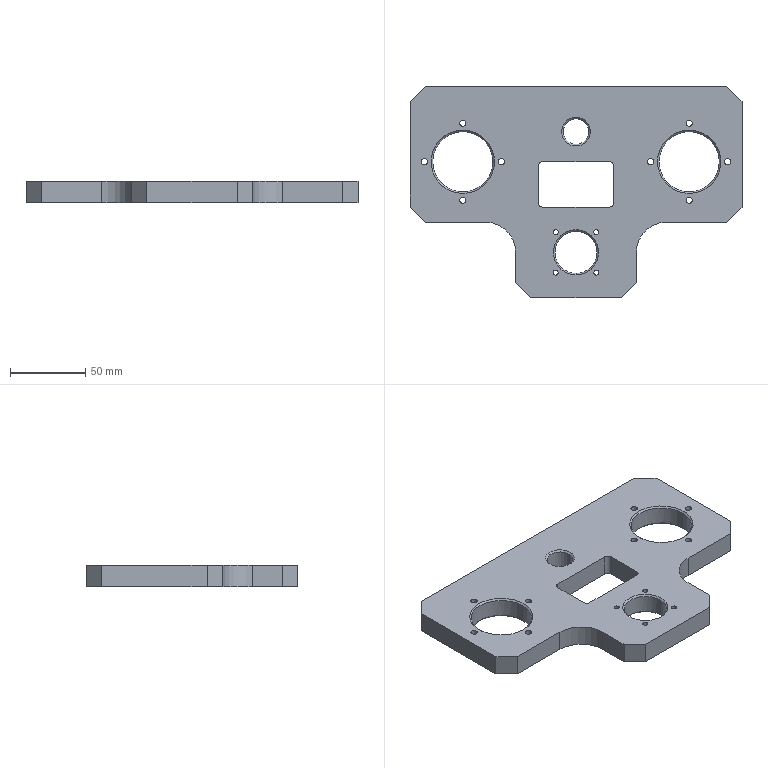Part | STEP file | fBY02F02M-00-06A | 1 solid | 74 faces | box 220 x 140 x 14 mm | volume 261096 mm3 | cylinder 38 | plane 20 | cone 16 | commonest cylinder face diameters 4.2 x16 3.3 x8 40 x6 6 x4 17 x2 28 x2